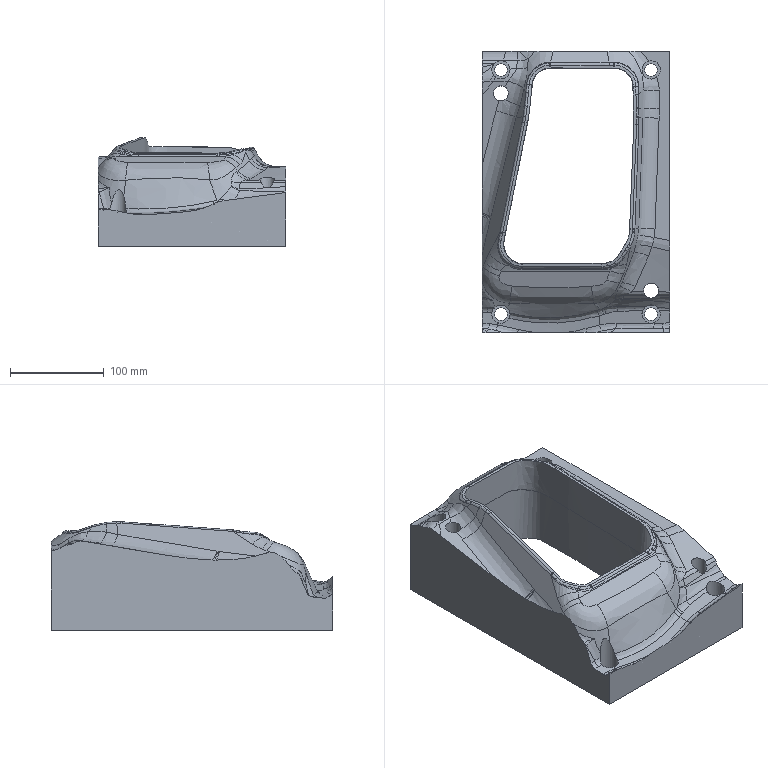Part | NX | features solid 2 | 1 solid | 213 faces | volume 2764791 mm3 | spline 194 | cylinder 10 | plane 9 | commonest cylinder face diameters 13.5 x4 19.5 x4 16 x2